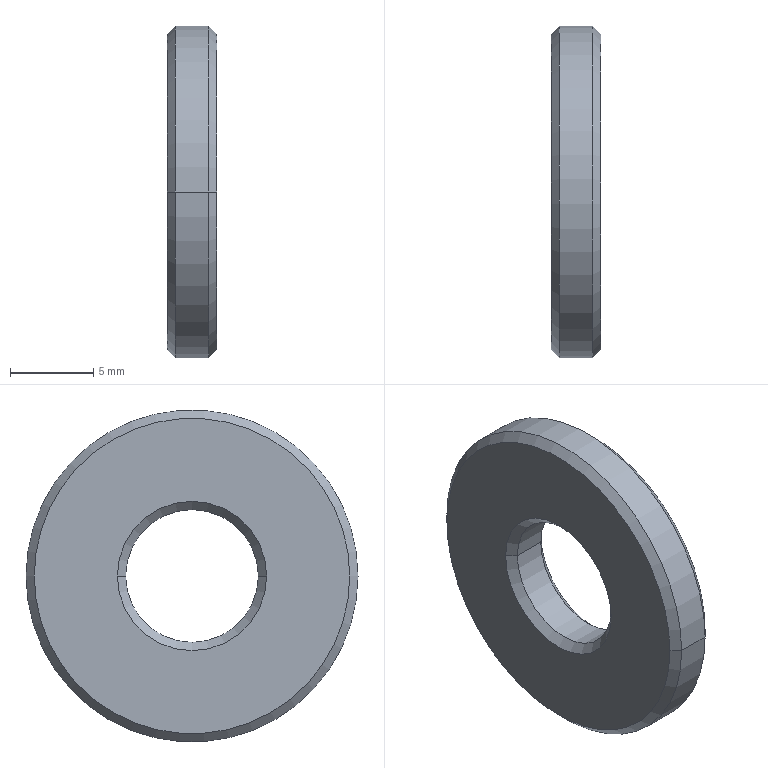Part | STEP file | wssm20_8_3_2_03 | 1 solid | 14 faces | box 3 x 20 x 20 mm | volume 769.69 mm3 | cone 8 | cylinder 4 | plane 2 | commonest cylinder face diameters 8 x2 20 x2
STEP:
#1=CARTESIAN_POINT('',(0.,0.,0.));
#2=DIRECTION('',(0.,0.,1.));
#3=DIRECTION('',(1.,0.,0.));
#4=AXIS2_PLACEMENT_3D('',#1,#2,#3);
#5=CARTESIAN_POINT('',(3.,9.5,0.));
#6=VERTEX_POINT('',#5);
#7=CARTESIAN_POINT('',(3.,-9.5,0.));
#8=VERTEX_POINT('',#7);
#9=CARTESIAN_POINT('',(3.,0.,0.));
#10=DIRECTION('',(1.,0.,0.));
#11=DIRECTION('',(0.,-1.,0.));
#12=AXIS2_PLACEMENT_3D('',#9,#10,#11);
#13=CIRCLE('',#12,9.5);
#14=CARTESIAN_POINT('',(2.5,0.,0.));
#15=DIRECTION('',(-1.,0.,0.));
#16=DIRECTION('',(0.,-1.,0.));
#17=AXIS2_PLACEMENT_3D('',#14,#15,#16);
#18=CONICAL_SURFACE('',#17,10.,0.7854);
#19=CARTESIAN_POINT('',(6.283,-0.5));
#20=DIRECTION('',(-1.,0.));
#21=VECTOR('',#20,1.);
#22=LINE('',#19,#21);
#23=(GEOMETRIC_REPRESENTATION_CONTEXT(2)PARAMETRIC_REPRESENTATION_CONTEXT()REPRESENTATION_CONTEXT('',''));
#24=DEFINITIONAL_REPRESENTATION('',(#22),#23);
#25=PCURVE('',#18,#24);
#26=CARTESIAN_POINT('',(3.,-7.,0.));
#27=DIRECTION('',(1.,0.,0.));
#28=DIRECTION('',(0.,0.,-1.));
#29=AXIS2_PLACEMENT_3D('',#26,#27,#28);
#30=PLANE('',#29);
#31=CARTESIAN_POINT('',(0.,7.));
#32=DIRECTION('',(0.,-1.));
#33=AXIS2_PLACEMENT_2D('',#31,#32);
#34=CIRCLE('',#33,9.5);
#35=(GEOMETRIC_REPRESENTATION_CONTEXT(2)PARAMETRIC_REPRESENTATION_CONTEXT()REPRESENTATION_CONTEXT('',''));
#36=DEFINITIONAL_REPRESENTATION('',(#34),#35);
#37=PCURVE('',#30,#36);
#38=SURFACE_CURVE('',#13,(#25,#37),.PCURVE_S1.);
#39=EDGE_CURVE('',#6,#8,#38,.T.);
#40=ORIENTED_EDGE('',*,*,#39,.F.);
#41=CARTESIAN_POINT('',(2.5,10.,0.));
#42=VERTEX_POINT('',#41);
#43=CARTESIAN_POINT('',(2.5,10.,0.));
#44=DIRECTION('',(-0.7071,0.7071,0.));
#45=VECTOR('',#44,1.);
#46=LINE('',#43,#45);
#47=CARTESIAN_POINT('',(3.142,0.));
#48=DIRECTION('',(0.,1.));
#49=VECTOR('',#48,1.);
#50=LINE('',#47,#49);
#51=(GEOMETRIC_REPRESENTATION_CONTEXT(2)PARAMETRIC_REPRESENTATION_CONTEXT()REPRESENTATION_CONTEXT('',''));
#52=DEFINITIONAL_REPRESENTATION('',(#50),#51);
#53=PCURVE('',#18,#52);
#54=CARTESIAN_POINT('',(2.5,0.,0.));
#55=DIRECTION('',(-1.,0.,0.));
#56=DIRECTION('',(0.,-1.,0.));
#57=AXIS2_PLACEMENT_3D('',#54,#55,#56);
#58=CONICAL_SURFACE('',#57,10.,0.7854);
#59=CARTESIAN_POINT('',(3.142,0.));
#60=DIRECTION('',(0.,1.));
#61=VECTOR('',#60,1.);
#62=LINE('',#59,#61);
#63=(GEOMETRIC_REPRESENTATION_CONTEXT(2)PARAMETRIC_REPRESENTATION_CONTEXT()REPRESENTATION_CONTEXT('',''));
#64=DEFINITIONAL_REPRESENTATION('',(#62),#63);
#65=PCURVE('',#58,#64);
#66=SURFACE_CURVE('',#46,(#53,#65),.PCURVE_S1.);
#67=EDGE_CURVE('',#6,#42,#66,.T.);
#68=ORIENTED_EDGE('',*,*,#67,.T.);
#69=CARTESIAN_POINT('',(2.5,-10.,0.));
#70=VERTEX_POINT('',#69);
#71=CARTESIAN_POINT('',(2.5,0.,0.));
#72=DIRECTION('',(1.,0.,0.));
#73=DIRECTION('',(0.,-1.,0.));
#74=AXIS2_PLACEMENT_3D('',#71,#72,#73);
#75=CIRCLE('',#74,10.);
#76=CARTESIAN_POINT('',(6.283,0.));
#77=DIRECTION('',(-1.,0.));
#78=VECTOR('',#77,1.);
#79=LINE('',#76,#78);
#80=(GEOMETRIC_REPRESENTATION_CONTEXT(2)PARAMETRIC_REPRESENTATION_CONTEXT()REPRESENTATION_CONTEXT('',''));
#81=DEFINITIONAL_REPRESENTATION('',(#79),#80);
#82=PCURVE('',#18,#81);
#83=CARTESIAN_POINT('',(1.5,0.,0.));
#84=DIRECTION('',(-1.,0.,0.));
#85=DIRECTION('',(0.,-1.,0.));
#86=AXIS2_PLACEMENT_3D('',#83,#84,#85);
#87=CYLINDRICAL_SURFACE('',#86,10.);
#88=CARTESIAN_POINT('',(6.283,-1.));
#89=DIRECTION('',(-1.,0.));
#90=VECTOR('',#89,1.);
#91=LINE('',#88,#90);
#92=(GEOMETRIC_REPRESENTATION_CONTEXT(2)PARAMETRIC_REPRESENTATION_CONTEXT()REPRESENTATION_CONTEXT('',''));
#93=DEFINITIONAL_REPRESENTATION('',(#91),#92);
#94=PCURVE('',#87,#93);
#95=SURFACE_CURVE('',#75,(#82,#94),.PCURVE_S1.);
#96=EDGE_CURVE('',#42,#70,#95,.T.);
#97=ORIENTED_EDGE('',*,*,#96,.T.);
#98=CARTESIAN_POINT('',(2.5,-10.,0.));
#99=DIRECTION('',(-0.7071,-0.7071,0.));
#100=VECTOR('',#99,1.);
#101=LINE('',#98,#100);
#102=CARTESIAN_POINT('',(0.,0.));
#103=DIRECTION('',(0.,1.));
#104=VECTOR('',#103,1.);
#105=LINE('',#102,#104);
#106=(GEOMETRIC_REPRESENTATION_CONTEXT(2)PARAMETRIC_REPRESENTATION_CONTEXT()REPRESENTATION_CONTEXT('',''));
#107=DEFINITIONAL_REPRESENTATION('',(#105),#106);
#108=PCURVE('',#18,#107);
#109=CARTESIAN_POINT('',(6.283,0.));
#110=DIRECTION('',(0.,1.));
#111=VECTOR('',#110,1.);
#112=LINE('',#109,#111);
#113=(GEOMETRIC_REPRESENTATION_CONTEXT(2)PARAMETRIC_REPRESENTATION_CONTEXT()REPRESENTATION_CONTEXT('',''));
#114=DEFINITIONAL_REPRESENTATION('',(#112),#113);
#115=PCURVE('',#58,#114);
#116=SURFACE_CURVE('',#101,(#108,#115),.PCURVE_S1.);
#117=EDGE_CURVE('',#8,#70,#116,.T.);
#118=ORIENTED_EDGE('',*,*,#117,.F.);
#119=EDGE_LOOP('',(#40,#68,#97,#118));
#120=FACE_BOUND('',#119,.T.);
#121=ADVANCED_FACE('',(#120),#18,.T.);
#122=CARTESIAN_POINT('',(2.5,-4.,0.));
#123=VERTEX_POINT('',#122);
#124=CARTESIAN_POINT('',(2.5,0.,-4.));
#125=VERTEX_POINT('',#124);
#126=CARTESIAN_POINT('',(2.5,0.,0.));
#127=DIRECTION('',(1.,0.,0.));
#128=DIRECTION('',(0.,-1.,0.));
#129=AXIS2_PLACEMENT_3D('',#126,#127,#128);
#130=CIRCLE('',#129,4.);
#131=CARTESIAN_POINT('',(3.,0.,0.));
#132=DIRECTION('',(1.,0.,0.));
#133=DIRECTION('',(0.,0.,-1.));
#134=AXIS2_PLACEMENT_3D('',#131,#132,#133);
#135=CONICAL_SURFACE('',#134,4.5,0.7854);
#136=CARTESIAN_POINT('',(4.712,-0.5));
#137=DIRECTION('',(1.,0.));
#138=VECTOR('',#137,1.);
#139=LINE('',#136,#138);
#140=(GEOMETRIC_REPRESENTATION_CONTEXT(2)PARAMETRIC_REPRESENTATION_CONTEXT()REPRESENTATION_CONTEXT('',''));
#141=DEFINITIONAL_REPRESENTATION('',(#139),#140);
#142=PCURVE('',#135,#141);
#143=CARTESIAN_POINT('',(1.5,0.,0.));
#144=DIRECTION('',(-1.,0.,0.));
#145=DIRECTION('',(0.,-1.,0.));
#146=AXIS2_PLACEMENT_3D('',#143,#144,#145);
#147=CYLINDRICAL_SURFACE('',#146,4.);
#148=CARTESIAN_POINT('',(6.283,-1.));
#149=DIRECTION('',(-1.,0.));
#150=VECTOR('',#149,1.);
#151=LINE('',#148,#150);
#152=(GEOMETRIC_REPRESENTATION_CONTEXT(2)PARAMETRIC_REPRESENTATION_CONTEXT()REPRESENTATION_CONTEXT('',''));
#153=DEFINITIONAL_REPRESENTATION('',(#151),#152);
#154=PCURVE('',#147,#153);
#155=SURFACE_CURVE('',#130,(#142,#154),.PCURVE_S1.);
#156=EDGE_CURVE('',#123,#125,#155,.T.);
#157=ORIENTED_EDGE('',*,*,#156,.T.);
#158=CARTESIAN_POINT('',(3.,0.,-4.5));
#159=VERTEX_POINT('',#158);
#160=CARTESIAN_POINT('',(3.,0.,-4.5));
#161=DIRECTION('',(0.7071,0.,-0.7071));
#162=VECTOR('',#161,1.);
#163=LINE('',#160,#162);
#164=CARTESIAN_POINT('',(6.283,0.));
#165=DIRECTION('',(0.,1.));
#166=VECTOR('',#165,1.);
#167=LINE('',#164,#166);
#168=(GEOMETRIC_REPRESENTATION_CONTEXT(2)PARAMETRIC_REPRESENTATION_CONTEXT()REPRESENTATION_CONTEXT('',''));
#169=DEFINITIONAL_REPRESENTATION('',(#167),#168);
#170=PCURVE('',#135,#169);
#171=CARTESIAN_POINT('',(3.,0.,0.));
#172=DIRECTION('',(1.,0.,0.));
#173=DIRECTION('',(0.,0.,-1.));
#174=AXIS2_PLACEMENT_3D('',#171,#172,#173);
#175=CONICAL_SURFACE('',#174,4.5,0.7854);
#176=CARTESIAN_POINT('',(0.,0.));
#177=DIRECTION('',(0.,1.));
#178=VECTOR('',#177,1.);
#179=LINE('',#176,#178);
#180=(GEOMETRIC_REPRESENTATION_CONTEXT(2)PARAMETRIC_REPRESENTATION_CONTEXT()REPRESENTATION_CONTEXT('',''));
#181=DEFINITIONAL_REPRESENTATION('',(#179),#180);
#182=PCURVE('',#175,#181);
#183=SURFACE_CURVE('',#163,(#170,#182),.PCURVE_S1.);
#184=EDGE_CURVE('',#125,#159,#183,.T.);
#185=ORIENTED_EDGE('',*,*,#184,.T.);
#186=CARTESIAN_POINT('',(3.,0.,4.5));
#187=VERTEX_POINT('',#186);
#188=CARTESIAN_POINT('',(3.,0.,0.));
#189=DIRECTION('',(-1.,0.,0.));
#190=DIRECTION('',(0.,0.,-1.));
#191=AXIS2_PLACEMENT_3D('',#188,#189,#190);
#192=CIRCLE('',#191,4.5);
#193=CARTESIAN_POINT('',(6.283,0.));
#194=DIRECTION('',(-1.,0.));
#195=VECTOR('',#194,1.);
#196=LINE('',#193,#195);
#197=(GEOMETRIC_REPRESENTATION_CONTEXT(2)PARAMETRIC_REPRESENTATION_CONTEXT()REPRESENTATION_CONTEXT('',''));
#198=DEFINITIONAL_REPRESENTATION('',(#196),#197);
#199=PCURVE('',#135,#198);
#200=CARTESIAN_POINT('',(4.5,7.));
#201=CARTESIAN_POINT('',(4.5,-0.7942));
#202=CARTESIAN_POINT('',(-2.25,3.103));
#203=CARTESIAN_POINT('',(-9.,7.));
#204=CARTESIAN_POINT('',(-2.25,10.897));
#205=CARTESIAN_POINT('',(4.5,14.794));
#206=CARTESIAN_POINT('',(4.5,7.));
#207=(BOUNDED_CURVE()B_SPLINE_CURVE(2,(#200,#201,#202,#203,#204,#205,#206),.UNSPECIFIED.,.T.,.F.)B_SPLINE_CURVE_WITH_KNOTS((1,2,2,2,2,1),(-2.094,0.,2.094,4.189,6.283,8.378),.UNSPECIFIED.)CURVE()GEOMETRIC_REPRESENTATION_ITEM()RATIONAL_B_SPLINE_CURVE((1.,0.5,1.,0.5,1.,0.5,1.))REPRESENTATION_ITEM(''));
#208=(GEOMETRIC_REPRESENTATION_CONTEXT(2)PARAMETRIC_REPRESENTATION_CONTEXT()REPRESENTATION_CONTEXT('',''));
#209=DEFINITIONAL_REPRESENTATION('',(#207),#208);
#210=PCURVE('',#30,#209);
#211=SURFACE_CURVE('',#192,(#199,#210),.PCURVE_S1.);
#212=EDGE_CURVE('',#159,#187,#211,.T.);
#213=ORIENTED_EDGE('',*,*,#212,.T.);
#214=CARTESIAN_POINT('',(2.5,0.,4.));
#215=VERTEX_POINT('',#214);
#216=CARTESIAN_POINT('',(3.,0.,4.5));
#217=DIRECTION('',(0.7071,0.,0.7071));
#218=VECTOR('',#217,1.);
#219=LINE('',#216,#218);
#220=CARTESIAN_POINT('',(3.142,0.));
#221=DIRECTION('',(0.,1.));
#222=VECTOR('',#221,1.);
#223=LINE('',#220,#222);
#224=(GEOMETRIC_REPRESENTATION_CONTEXT(2)PARAMETRIC_REPRESENTATION_CONTEXT()REPRESENTATION_CONTEXT('',''));
#225=DEFINITIONAL_REPRESENTATION('',(#223),#224);
#226=PCURVE('',#135,#225);
#227=CARTESIAN_POINT('',(3.142,0.));
#228=DIRECTION('',(0.,1.));
#229=VECTOR('',#228,1.);
#230=LINE('',#227,#229);
#231=(GEOMETRIC_REPRESENTATION_CONTEXT(2)PARAMETRIC_REPRESENTATION_CONTEXT()REPRESENTATION_CONTEXT('',''));
#232=DEFINITIONAL_REPRESENTATION('',(#230),#231);
#233=PCURVE('',#175,#232);
#234=SURFACE_CURVE('',#219,(#226,#233),.PCURVE_S1.);
#235=EDGE_CURVE('',#215,#187,#234,.T.);
#236=ORIENTED_EDGE('',*,*,#235,.F.);
#237=CARTESIAN_POINT('',(2.5,0.,0.));
#238=DIRECTION('',(1.,0.,0.));
#239=DIRECTION('',(0.,-1.,0.));
#240=AXIS2_PLACEMENT_3D('',#237,#238,#239);
#241=CIRCLE('',#240,4.);
#242=CARTESIAN_POINT('',(-1.571,-0.5));
#243=DIRECTION('',(1.,0.));
#244=VECTOR('',#243,1.);
#245=LINE('',#242,#244);
#246=(GEOMETRIC_REPRESENTATION_CONTEXT(2)PARAMETRIC_REPRESENTATION_CONTEXT()REPRESENTATION_CONTEXT('',''));
#247=DEFINITIONAL_REPRESENTATION('',(#245),#246);
#248=PCURVE('',#135,#247);
#249=CARTESIAN_POINT('',(1.5,0.,0.));
#250=DIRECTION('',(-1.,0.,0.));
#251=DIRECTION('',(0.,-1.,0.));
#252=AXIS2_PLACEMENT_3D('',#249,#250,#251);
#253=CYLINDRICAL_SURFACE('',#252,4.);
#254=CARTESIAN_POINT('',(6.283,-1.));
#255=DIRECTION('',(-1.,0.));
#256=VECTOR('',#255,1.);
#257=LINE('',#254,#256);
#258=(GEOMETRIC_REPRESENTATION_CONTEXT(2)PARAMETRIC_REPRESENTATION_CONTEXT()REPRESENTATION_CONTEXT('',''));
#259=DEFINITIONAL_REPRESENTATION('',(#257),#258);
#260=PCURVE('',#253,#259);
#261=SURFACE_CURVE('',#241,(#248,#260),.PCURVE_S1.);
#262=EDGE_CURVE('',#215,#123,#261,.T.);
#263=ORIENTED_EDGE('',*,*,#262,.T.);
#264=EDGE_LOOP('',(#157,#185,#213,#236,#263));
#265=FACE_BOUND('',#264,.F.);
#266=ADVANCED_FACE('',(#265),#135,.F.);
#267=ORIENTED_EDGE('',*,*,#96,.F.);
#268=CARTESIAN_POINT('',(0.5,10.,0.));
#269=VERTEX_POINT('',#268);
#270=CARTESIAN_POINT('',(1.5,10.,0.));
#271=DIRECTION('',(-1.,0.,0.));
#272=VECTOR('',#271,1.);
#273=LINE('',#270,#272);
#274=CARTESIAN_POINT('',(3.142,0.));
#275=DIRECTION('',(0.,1.));
#276=VECTOR('',#275,1.);
#277=LINE('',#274,#276);
#278=(GEOMETRIC_REPRESENTATION_CONTEXT(2)PARAMETRIC_REPRESENTATION_CONTEXT()REPRESENTATION_CONTEXT('',''));
#279=DEFINITIONAL_REPRESENTATION('',(#277),#278);
#280=PCURVE('',#87,#279);
#281=CARTESIAN_POINT('',(1.5,0.,0.));
#282=DIRECTION('',(-1.,0.,0.));
#283=DIRECTION('',(0.,-1.,0.));
#284=AXIS2_PLACEMENT_3D('',#281,#282,#283);
#285=CYLINDRICAL_SURFACE('',#284,10.);
#286=CARTESIAN_POINT('',(3.142,0.));
#287=DIRECTION('',(0.,1.));
#288=VECTOR('',#287,1.);
#289=LINE('',#286,#288);
#290=(GEOMETRIC_REPRESENTATION_CONTEXT(2)PARAMETRIC_REPRESENTATION_CONTEXT()REPRESENTATION_CONTEXT('',''));
#291=DEFINITIONAL_REPRESENTATION('',(#289),#290);
#292=PCURVE('',#285,#291);
#293=SURFACE_CURVE('',#273,(#280,#292),.PCURVE_S1.);
#294=EDGE_CURVE('',#42,#269,#293,.T.);
#295=ORIENTED_EDGE('',*,*,#294,.T.);
#296=CARTESIAN_POINT('',(0.5,-10.,0.));
#297=VERTEX_POINT('',#296);
#298=CARTESIAN_POINT('',(0.5,0.,0.));
#299=DIRECTION('',(1.,0.,0.));
#300=DIRECTION('',(0.,-1.,0.));
#301=AXIS2_PLACEMENT_3D('',#298,#299,#300);
#302=CIRCLE('',#301,10.);
#303=CARTESIAN_POINT('',(6.283,1.));
#304=DIRECTION('',(-1.,0.));
#305=VECTOR('',#304,1.);
#306=LINE('',#303,#305);
#307=(GEOMETRIC_REPRESENTATION_CONTEXT(2)PARAMETRIC_REPRESENTATION_CONTEXT()REPRESENTATION_CONTEXT('',''));
#308=DEFINITIONAL_REPRESENTATION('',(#306),#307);
#309=PCURVE('',#87,#308);
#310=CARTESIAN_POINT('',(0.5,0.,0.));
#311=DIRECTION('',(1.,0.,0.));
#312=DIRECTION('',(0.,1.,0.));
#313=AXIS2_PLACEMENT_3D('',#310,#311,#312);
#314=CONICAL_SURFACE('',#313,10.,0.7854);
#315=CARTESIAN_POINT('',(-3.142,0.));
#316=DIRECTION('',(1.,0.));
#317=VECTOR('',#316,1.);
#318=LINE('',#315,#317);
#319=(GEOMETRIC_REPRESENTATION_CONTEXT(2)PARAMETRIC_REPRESENTATION_CONTEXT()REPRESENTATION_CONTEXT('',''));
#320=DEFINITIONAL_REPRESENTATION('',(#318),#319);
#321=PCURVE('',#314,#320);
#322=SURFACE_CURVE('',#302,(#309,#321),.PCURVE_S1.);
#323=EDGE_CURVE('',#269,#297,#322,.T.);
#324=ORIENTED_EDGE('',*,*,#323,.T.);
#325=CARTESIAN_POINT('',(1.5,-10.,0.));
#326=DIRECTION('',(-1.,0.,0.));
#327=VECTOR('',#326,1.);
#328=LINE('',#325,#327);
#329=CARTESIAN_POINT('',(0.,0.));
#330=DIRECTION('',(0.,1.));
#331=VECTOR('',#330,1.);
#332=LINE('',#329,#331);
#333=(GEOMETRIC_REPRESENTATION_CONTEXT(2)PARAMETRIC_REPRESENTATION_CONTEXT()REPRESENTATION_CONTEXT('',''));
#334=DEFINITIONAL_REPRESENTATION('',(#332),#333);
#335=PCURVE('',#87,#334);
#336=CARTESIAN_POINT('',(6.283,0.));
#337=DIRECTION('',(0.,1.));
#338=VECTOR('',#337,1.);
#339=LINE('',#336,#338);
#340=(GEOMETRIC_REPRESENTATION_CONTEXT(2)PARAMETRIC_REPRESENTATION_CONTEXT()REPRESENTATION_CONTEXT('',''));
#341=DEFINITIONAL_REPRESENTATION('',(#339),#340);
#342=PCURVE('',#285,#341);
#343=SURFACE_CURVE('',#328,(#335,#342),.PCURVE_S1.);
#344=EDGE_CURVE('',#70,#297,#343,.T.);
#345=ORIENTED_EDGE('',*,*,#344,.F.);
#346=EDGE_LOOP('',(#267,#295,#324,#345));
#347=FACE_BOUND('',#346,.T.);
#348=ADVANCED_FACE('',(#347),#87,.T.);
#349=CARTESIAN_POINT('',(0.5,-4.,0.));
#350=VERTEX_POINT('',#349);
#351=CARTESIAN_POINT('',(1.5,-4.,0.));
#352=DIRECTION('',(-1.,0.,0.));
#353=VECTOR('',#352,1.);
#354=LINE('',#351,#353);
#355=CARTESIAN_POINT('',(6.283,0.));
#356=DIRECTION('',(0.,1.));
#357=VECTOR('',#356,1.);
#358=LINE('',#355,#357);
#359=(GEOMETRIC_REPRESENTATION_CONTEXT(2)PARAMETRIC_REPRESENTATION_CONTEXT()REPRESENTATION_CONTEXT('',''));
#360=DEFINITIONAL_REPRESENTATION('',(#358),#359);
#361=PCURVE('',#147,#360);
#362=CARTESIAN_POINT('',(0.,0.));
#363=DIRECTION('',(0.,1.));
#364=VECTOR('',#363,1.);
#365=LINE('',#362,#364);
#366=(GEOMETRIC_REPRESENTATION_CONTEXT(2)PARAMETRIC_REPRESENTATION_CONTEXT()REPRESENTATION_CONTEXT('',''));
#367=DEFINITIONAL_REPRESENTATION('',(#365),#366);
#368=PCURVE('',#253,#367);
#369=SURFACE_CURVE('',#354,(#361,#368),.PCURVE_S1.);
#370=EDGE_CURVE('',#123,#350,#369,.T.);
#371=ORIENTED_EDGE('',*,*,#370,.T.);
#372=CARTESIAN_POINT('',(0.5,4.,0.));
#373=VERTEX_POINT('',#372);
#374=CARTESIAN_POINT('',(0.5,0.,0.));
#375=DIRECTION('',(1.,0.,0.));
#376=DIRECTION('',(0.,-1.,0.));
#377=AXIS2_PLACEMENT_3D('',#374,#375,#376);
#378=CIRCLE('',#377,4.);
#379=CARTESIAN_POINT('',(6.283,1.));
#380=DIRECTION('',(-1.,0.));
#381=VECTOR('',#380,1.);
#382=LINE('',#379,#381);
#383=(GEOMETRIC_REPRESENTATION_CONTEXT(2)PARAMETRIC_REPRESENTATION_CONTEXT()REPRESENTATION_CONTEXT('',''));
#384=DEFINITIONAL_REPRESENTATION('',(#382),#383);
#385=PCURVE('',#147,#384);
#386=CARTESIAN_POINT('',(0.,0.,0.));
#387=DIRECTION('',(-1.,0.,0.));
#388=DIRECTION('',(0.,-1.,0.));
#389=AXIS2_PLACEMENT_3D('',#386,#387,#388);
#390=CONICAL_SURFACE('',#389,4.5,0.7854);
#391=CARTESIAN_POINT('',(6.283,-0.5));
#392=DIRECTION('',(-1.,0.));
#393=VECTOR('',#392,1.);
#394=LINE('',#391,#393);
#395=(GEOMETRIC_REPRESENTATION_CONTEXT(2)PARAMETRIC_REPRESENTATION_CONTEXT()REPRESENTATION_CONTEXT('',''));
#396=DEFINITIONAL_REPRESENTATION('',(#394),#395);
#397=PCURVE('',#390,#396);
#398=SURFACE_CURVE('',#378,(#385,#397),.PCURVE_S1.);
#399=EDGE_CURVE('',#350,#373,#398,.T.);
#400=ORIENTED_EDGE('',*,*,#399,.T.);
#401=CARTESIAN_POINT('',(2.5,4.,0.));
#402=VERTEX_POINT('',#401);
#403=CARTESIAN_POINT('',(1.5,4.,0.));
#404=DIRECTION('',(-1.,0.,0.));
#405=VECTOR('',#404,1.);
#406=LINE('',#403,#405);
#407=CARTESIAN_POINT('',(3.142,0.));
#408=DIRECTION('',(0.,1.));
#409=VECTOR('',#408,1.);
#410=LINE('',#407,#409);
#411=(GEOMETRIC_REPRESENTATION_CONTEXT(2)PARAMETRIC_REPRESENTATION_CONTEXT()REPRESENTATION_CONTEXT('',''));
#412=DEFINITIONAL_REPRESENTATION('',(#410),#411);
#413=PCURVE('',#147,#412);
#414=CARTESIAN_POINT('',(3.142,0.));
#415=DIRECTION('',(0.,1.));
#416=VECTOR('',#415,1.);
#417=LINE('',#414,#416);
#418=(GEOMETRIC_REPRESENTATION_CONTEXT(2)PARAMETRIC_REPRESENTATION_CONTEXT()REPRESENTATION_CONTEXT('',''));
#419=DEFINITIONAL_REPRESENTATION('',(#417),#418);
#420=PCURVE('',#253,#419);
#421=SURFACE_CURVE('',#406,(#413,#420),.PCURVE_S1.);
#422=EDGE_CURVE('',#402,#373,#421,.T.);
#423=ORIENTED_EDGE('',*,*,#422,.F.);
#424=CARTESIAN_POINT('',(2.5,0.,0.));
#425=DIRECTION('',(1.,0.,0.));
#426=DIRECTION('',(0.,-1.,0.));
#427=AXIS2_PLACEMENT_3D('',#424,#425,#426);
#428=CIRCLE('',#427,4.);
#429=CARTESIAN_POINT('',(6.283,-1.));
#430=DIRECTION('',(-1.,0.));
#431=VECTOR('',#430,1.);
#432=LINE('',#429,#431);
#433=(GEOMETRIC_REPRESENTATION_CONTEXT(2)PARAMETRIC_REPRESENTATION_CONTEXT()REPRESENTATION_CONTEXT('',''));
#434=DEFINITIONAL_REPRESENTATION('',(#432),#433);
#435=PCURVE('',#147,#434);
#436=CARTESIAN_POINT('',(-1.571,-0.5));
#437=DIRECTION('',(1.,0.));
#438=VECTOR('',#437,1.);
#439=LINE('',#436,#438);
#440=(GEOMETRIC_REPRESENTATION_CONTEXT(2)PARAMETRIC_REPRESENTATION_CONTEXT()REPRESENTATION_CONTEXT('',''));
#441=DEFINITIONAL_REPRESENTATION('',(#439),#440);
#442=PCURVE('',#175,#441);
#443=SURFACE_CURVE('',#428,(#435,#442),.PCURVE_S1.);
#444=EDGE_CURVE('',#125,#402,#443,.T.);
#445=ORIENTED_EDGE('',*,*,#444,.F.);
#446=ORIENTED_EDGE('',*,*,#156,.F.);
#447=EDGE_LOOP('',(#371,#400,#423,#445,#446));
#448=FACE_BOUND('',#447,.F.);
#449=ADVANCED_FACE('',(#448),#147,.F.);
#450=CARTESIAN_POINT('',(0.,9.5,0.));
#451=VERTEX_POINT('',#450);
#452=CARTESIAN_POINT('',(0.,-9.5,0.));
#453=VERTEX_POINT('',#452);
#454=CARTESIAN_POINT('',(0.,0.,0.));
#455=DIRECTION('',(1.,0.,0.));
#456=DIRECTION('',(0.,1.,0.));
#457=AXIS2_PLACEMENT_3D('',#454,#455,#456);
#458=CIRCLE('',#457,9.5);
#459=CARTESIAN_POINT('',(0.,-0.5));
#460=DIRECTION('',(1.,0.));
#461=VECTOR('',#460,1.);
#462=LINE('',#459,#461);
#463=(GEOMETRIC_REPRESENTATION_CONTEXT(2)PARAMETRIC_REPRESENTATION_CONTEXT()REPRESENTATION_CONTEXT('',''));
#464=DEFINITIONAL_REPRESENTATION('',(#462),#463);
#465=PCURVE('',#314,#464);
#466=CARTESIAN_POINT('',(0.,-7.,0.));
#467=DIRECTION('',(-1.,0.,0.));
#468=DIRECTION('',(0.,-1.,0.));
#469=AXIS2_PLACEMENT_3D('',#466,#467,#468);
#470=PLANE('',#469);
#471=CARTESIAN_POINT('',(-16.5,0.));
#472=CARTESIAN_POINT('',(-16.5,16.454));
#473=CARTESIAN_POINT('',(-2.25,8.227));
#474=CARTESIAN_POINT('',(12.,0.));
#475=CARTESIAN_POINT('',(-2.25,-8.227));
#476=CARTESIAN_POINT('',(-16.5,-16.454));
#477=CARTESIAN_POINT('',(-16.5,0.));
#478=(BOUNDED_CURVE()B_SPLINE_CURVE(2,(#471,#472,#473,#474,#475,#476,#477),.UNSPECIFIED.,.T.,.F.)B_SPLINE_CURVE_WITH_KNOTS((1,2,2,2,2,1),(-2.094,0.,2.094,4.189,6.283,8.378),.UNSPECIFIED.)CURVE()GEOMETRIC_REPRESENTATION_ITEM()RATIONAL_B_SPLINE_CURVE((1.,0.5,1.,0.5,1.,0.5,1.))REPRESENTATION_ITEM(''));
#479=(GEOMETRIC_REPRESENTATION_CONTEXT(2)PARAMETRIC_REPRESENTATION_CONTEXT()REPRESENTATION_CONTEXT('',''));
#480=DEFINITIONAL_REPRESENTATION('',(#478),#479);
#481=PCURVE('',#470,#480);
#482=SURFACE_CURVE('',#458,(#465,#481),.PCURVE_S1.);
#483=EDGE_CURVE('',#451,#453,#482,.T.);
#484=ORIENTED_EDGE('',*,*,#483,.T.);
#485=CARTESIAN_POINT('',(0.5,-10.,0.));
#486=DIRECTION('',(0.7071,-0.7071,0.));
#487=VECTOR('',#486,1.);
#488=LINE('',#485,#487);
#489=CARTESIAN_POINT('',(3.142,0.));
#490=DIRECTION('',(0.,1.));
#491=VECTOR('',#490,1.);
#492=LINE('',#489,#491);
#493=(GEOMETRIC_REPRESENTATION_CONTEXT(2)PARAMETRIC_REPRESENTATION_CONTEXT()REPRESENTATION_CONTEXT('',''));
#494=DEFINITIONAL_REPRESENTATION('',(#492),#493);
#495=PCURVE('',#314,#494);
#496=CARTESIAN_POINT('',(0.5,0.,0.));
#497=DIRECTION('',(1.,0.,0.));
#498=DIRECTION('',(0.,1.,0.));
#499=AXIS2_PLACEMENT_3D('',#496,#497,#498);
#500=CONICAL_SURFACE('',#499,10.,0.7854);
#501=CARTESIAN_POINT('',(3.142,0.));
#502=DIRECTION('',(0.,1.));
#503=VECTOR('',#502,1.);
#504=LINE('',#501,#503);
#505=(GEOMETRIC_REPRESENTATION_CONTEXT(2)PARAMETRIC_REPRESENTATION_CONTEXT()REPRESENTATION_CONTEXT('',''));
#506=DEFINITIONAL_REPRESENTATION('',(#504),#505);
#507=PCURVE('',#500,#506);
#508=SURFACE_CURVE('',#488,(#495,#507),.PCURVE_S1.);
#509=EDGE_CURVE('',#453,#297,#508,.T.);
#510=ORIENTED_EDGE('',*,*,#509,.T.);
#511=ORIENTED_EDGE('',*,*,#323,.F.);
#512=CARTESIAN_POINT('',(0.5,10.,0.));
#513=DIRECTION('',(0.7071,0.7071,0.));
#514=VECTOR('',#513,1.);
#515=LINE('',#512,#514);
#516=CARTESIAN_POINT('',(0.,0.));
#517=DIRECTION('',(0.,1.));
#518=VECTOR('',#517,1.);
#519=LINE('',#516,#518);
#520=(GEOMETRIC_REPRESENTATION_CONTEXT(2)PARAMETRIC_REPRESENTATION_CONTEXT()REPRESENTATION_CONTEXT('',''));
#521=DEFINITIONAL_REPRESENTATION('',(#519),#520);
#522=PCURVE('',#314,#521);
#523=CARTESIAN_POINT('',(6.283,0.));
#524=DIRECTION('',(0.,1.));
#525=VECTOR('',#524,1.);
#526=LINE('',#523,#525);
#527=(GEOMETRIC_REPRESENTATION_CONTEXT(2)PARAMETRIC_REPRESENTATION_CONTEXT()REPRESENTATION_CONTEXT('',''));
#528=DEFINITIONAL_REPRESENTATION('',(#526),#527);
#529=PCURVE('',#500,#528);
#530=SURFACE_CURVE('',#515,(#522,#529),.PCURVE_S1.);
#531=EDGE_CURVE('',#451,#269,#530,.T.);
#532=ORIENTED_EDGE('',*,*,#531,.F.);
#533=EDGE_LOOP('',(#484,#510,#511,#532));
#534=FACE_BOUND('',#533,.T.);
#535=ADVANCED_FACE('',(#534),#314,.T.);
#536=CARTESIAN_POINT('',(0.,-4.5,0.));
#537=VERTEX_POINT('',#536);
#538=CARTESIAN_POINT('',(0.,-4.5,0.));
#539=DIRECTION('',(-0.7071,-0.7071,0.));
#540=VECTOR('',#539,1.);
#541=LINE('',#538,#540);
#542=CARTESIAN_POINT('',(6.283,0.));
#543=DIRECTION('',(0.,1.));
#544=VECTOR('',#543,1.);
#545=LINE('',#542,#544);
#546=(GEOMETRIC_REPRESENTATION_CONTEXT(2)PARAMETRIC_REPRESENTATION_CONTEXT()REPRESENTATION_CONTEXT('',''));
#547=DEFINITIONAL_REPRESENTATION('',(#545),#546);
#548=PCURVE('',#390,#547);
#549=CARTESIAN_POINT('',(0.,0.,0.));
#550=DIRECTION('',(-1.,0.,0.));
#551=DIRECTION('',(0.,-1.,0.));
#552=AXIS2_PLACEMENT_3D('',#549,#550,#551);
#553=CONICAL_SURFACE('',#552,4.5,0.7854);
#554=CARTESIAN_POINT('',(0.,0.));
#555=DIRECTION('',(0.,1.));
#556=VECTOR('',#555,1.);
#557=LINE('',#554,#556);
#558=(GEOMETRIC_REPRESENTATION_CONTEXT(2)PARAMETRIC_REPRESENTATION_CONTEXT()REPRESENTATION_CONTEXT('',''));
#559=DEFINITIONAL_REPRESENTATION('',(#557),#558);
#560=PCURVE('',#553,#559);
#561=SURFACE_CURVE('',#541,(#548,#560),.PCURVE_S1.);
#562=EDGE_CURVE('',#350,#537,#561,.T.);
#563=ORIENTED_EDGE('',*,*,#562,.T.);
#564=CARTESIAN_POINT('',(0.,4.5,0.));
#565=VERTEX_POINT('',#564);
#566=CARTESIAN_POINT('',(0.,0.,0.));
#567=DIRECTION('',(1.,0.,0.));
#568=DIRECTION('',(0.,-1.,0.));
#569=AXIS2_PLACEMENT_3D('',#566,#567,#568);
#570=CIRCLE('',#569,4.5);
#571=CARTESIAN_POINT('',(6.283,0.));
#572=DIRECTION('',(-1.,0.));
#573=VECTOR('',#572,1.);
#574=LINE('',#571,#573);
#575=(GEOMETRIC_REPRESENTATION_CONTEXT(2)PARAMETRIC_REPRESENTATION_CONTEXT()REPRESENTATION_CONTEXT('',''));
#576=DEFINITIONAL_REPRESENTATION('',(#574),#575);
#577=PCURVE('',#390,#576);
#578=CARTESIAN_POINT('',(-2.5,0.));
#579=CARTESIAN_POINT('',(-2.5,-7.794));
#580=CARTESIAN_POINT('',(-9.25,-3.897));
#581=CARTESIAN_POINT('',(-16.,0.));
#582=CARTESIAN_POINT('',(-9.25,3.897));
#583=CARTESIAN_POINT('',(-2.5,7.794));
#584=CARTESIAN_POINT('',(-2.5,0.));
#585=(BOUNDED_CURVE()B_SPLINE_CURVE(2,(#578,#579,#580,#581,#582,#583,#584),.UNSPECIFIED.,.T.,.F.)B_SPLINE_CURVE_WITH_KNOTS((1,2,2,2,2,1),(-2.094,0.,2.094,4.189,6.283,8.378),.UNSPECIFIED.)CURVE()GEOMETRIC_REPRESENTATION_ITEM()RATIONAL_B_SPLINE_CURVE((1.,0.5,1.,0.5,1.,0.5,1.))REPRESENTATION_ITEM(''));
#586=(GEOMETRIC_REPRESENTATION_CONTEXT(2)PARAMETRIC_REPRESENTATION_CONTEXT()REPRESENTATION_CONTEXT('',''));
#587=DEFINITIONAL_REPRESENTATION('',(#585),#586);
#588=PCURVE('',#470,#587);
#589=SURFACE_CURVE('',#570,(#577,#588),.PCURVE_S1.);
#590=EDGE_CURVE('',#537,#565,#589,.T.);
#591=ORIENTED_EDGE('',*,*,#590,.T.);
#592=CARTESIAN_POINT('',(0.,4.5,0.));
#593=DIRECTION('',(-0.7071,0.7071,0.));
#594=VECTOR('',#593,1.);
#595=LINE('',#592,#594);
#596=CARTESIAN_POINT('',(3.142,0.));
#597=DIRECTION('',(0.,1.));
#598=VECTOR('',#597,1.);
#599=LINE('',#596,#598);
#600=(GEOMETRIC_REPRESENTATION_CONTEXT(2)PARAMETRIC_REPRESENTATION_CONTEXT()REPRESENTATION_CONTEXT('',''));
#601=DEFINITIONAL_REPRESENTATION('',(#599),#600);
#602=PCURVE('',#390,#601);
#603=CARTESIAN_POINT('',(3.142,0.));
#604=DIRECTION('',(0.,1.));
#605=VECTOR('',#604,1.);
#606=LINE('',#603,#605);
#607=(GEOMETRIC_REPRESENTATION_CONTEXT(2)PARAMETRIC_REPRESENTATION_CONTEXT()REPRESENTATION_CONTEXT('',''));
#608=DEFINITIONAL_REPRESENTATION('',(#606),#607);
#609=PCURVE('',#553,#608);
#610=SURFACE_CURVE('',#595,(#602,#609),.PCURVE_S1.);
#611=EDGE_CURVE('',#373,#565,#610,.T.);
#612=ORIENTED_EDGE('',*,*,#611,.F.);
#613=ORIENTED_EDGE('',*,*,#399,.F.);
#614=EDGE_LOOP('',(#563,#591,#612,#613));
#615=FACE_BOUND('',#614,.F.);
#616=ADVANCED_FACE('',(#615),#390,.F.);
#617=CARTESIAN_POINT('',(3.,0.,0.));
#618=DIRECTION('',(1.,0.,0.));
#619=DIRECTION('',(0.,-1.,0.));
#620=AXIS2_PLACEMENT_3D('',#617,#618,#619);
#621=CIRCLE('',#620,9.5);
#622=CARTESIAN_POINT('',(0.,7.));
#623=DIRECTION('',(0.,-1.));
#624=AXIS2_PLACEMENT_2D('',#622,#623);
#625=CIRCLE('',#624,9.5);
#626=(GEOMETRIC_REPRESENTATION_CONTEXT(2)PARAMETRIC_REPRESENTATION_CONTEXT()REPRESENTATION_CONTEXT('',''));
#627=DEFINITIONAL_REPRESENTATION('',(#625),#626);
#628=PCURVE('',#30,#627);
#629=CARTESIAN_POINT('',(6.283,-0.5));
#630=DIRECTION('',(-1.,0.));
#631=VECTOR('',#630,1.);
#632=LINE('',#629,#631);
#633=(GEOMETRIC_REPRESENTATION_CONTEXT(2)PARAMETRIC_REPRESENTATION_CONTEXT()REPRESENTATION_CONTEXT('',''));
#634=DEFINITIONAL_REPRESENTATION('',(#632),#633);
#635=PCURVE('',#58,#634);
#636=SURFACE_CURVE('',#621,(#628,#635),.PCURVE_S1.);
#637=EDGE_CURVE('',#8,#6,#636,.T.);
#638=ORIENTED_EDGE('',*,*,#637,.T.);
#639=ORIENTED_EDGE('',*,*,#39,.T.);
#640=EDGE_LOOP('',(#638,#639));
#641=FACE_BOUND('',#640,.T.);
#642=ORIENTED_EDGE('',*,*,#212,.T.);
#643=CARTESIAN_POINT('',(3.,0.,0.));
#644=DIRECTION('',(-1.,0.,0.));
#645=DIRECTION('',(0.,0.,-1.));
#646=AXIS2_PLACEMENT_3D('',#643,#644,#645);
#647=CIRCLE('',#646,4.5);
#648=CARTESIAN_POINT('',(4.5,7.));
#649=CARTESIAN_POINT('',(4.5,-0.7942));
#650=CARTESIAN_POINT('',(-2.25,3.103));
#651=CARTESIAN_POINT('',(-9.,7.));
#652=CARTESIAN_POINT('',(-2.25,10.897));
#653=CARTESIAN_POINT('',(4.5,14.794));
#654=CARTESIAN_POINT('',(4.5,7.));
#655=(BOUNDED_CURVE()B_SPLINE_CURVE(2,(#648,#649,#650,#651,#652,#653,#654),.UNSPECIFIED.,.T.,.F.)B_SPLINE_CURVE_WITH_KNOTS((1,2,2,2,2,1),(-2.094,0.,2.094,4.189,6.283,8.378),.UNSPECIFIED.)CURVE()GEOMETRIC_REPRESENTATION_ITEM()RATIONAL_B_SPLINE_CURVE((1.,0.5,1.,0.5,1.,0.5,1.))REPRESENTATION_ITEM(''));
#656=(GEOMETRIC_REPRESENTATION_CONTEXT(2)PARAMETRIC_REPRESENTATION_CONTEXT()REPRESENTATION_CONTEXT('',''));
#657=DEFINITIONAL_REPRESENTATION('',(#655),#656);
#658=PCURVE('',#30,#657);
#659=CARTESIAN_POINT('',(6.283,0.));
#660=DIRECTION('',(-1.,0.));
#661=VECTOR('',#660,1.);
#662=LINE('',#659,#661);
#663=(GEOMETRIC_REPRESENTATION_CONTEXT(2)PARAMETRIC_REPRESENTATION_CONTEXT()REPRESENTATION_CONTEXT('',''));
#664=DEFINITIONAL_REPRESENTATION('',(#662),#663);
#665=PCURVE('',#175,#664);
#666=SURFACE_CURVE('',#647,(#658,#665),.PCURVE_S1.);
#667=EDGE_CURVE('',#187,#159,#666,.T.);
#668=ORIENTED_EDGE('',*,*,#667,.T.);
#669=EDGE_LOOP('',(#642,#668));
#670=FACE_BOUND('',#669,.T.);
#671=ADVANCED_FACE('',(#641,#670),#30,.T.);
#672=ORIENTED_EDGE('',*,*,#67,.F.);
#673=ORIENTED_EDGE('',*,*,#637,.F.);
#674=ORIENTED_EDGE('',*,*,#117,.T.);
#675=CARTESIAN_POINT('',(2.5,0.,0.));
#676=DIRECTION('',(1.,0.,0.));
#677=DIRECTION('',(0.,-1.,0.));
#678=AXIS2_PLACEMENT_3D('',#675,#676,#677);
#679=CIRCLE('',#678,10.);
#680=CARTESIAN_POINT('',(6.283,0.));
#681=DIRECTION('',(-1.,0.));
#682=VECTOR('',#681,1.);
#683=LINE('',#680,#682);
#684=(GEOMETRIC_REPRESENTATION_CONTEXT(2)PARAMETRIC_REPRESENTATION_CONTEXT()REPRESENTATION_CONTEXT('',''));
#685=DEFINITIONAL_REPRESENTATION('',(#683),#684);
#686=PCURVE('',#58,#685);
#687=CARTESIAN_POINT('',(6.283,-1.));
#688=DIRECTION('',(-1.,0.));
#689=VECTOR('',#688,1.);
#690=LINE('',#687,#689);
#691=(GEOMETRIC_REPRESENTATION_CONTEXT(2)PARAMETRIC_REPRESENTATION_CONTEXT()REPRESENTATION_CONTEXT('',''));
#692=DEFINITIONAL_REPRESENTATION('',(#690),#691);
#693=PCURVE('',#285,#692);
#694=SURFACE_CURVE('',#679,(#686,#693),.PCURVE_S1.);
#695=EDGE_CURVE('',#70,#42,#694,.T.);
#696=ORIENTED_EDGE('',*,*,#695,.T.);
#697=EDGE_LOOP('',(#672,#673,#674,#696));
#698=FACE_BOUND('',#697,.T.);
#699=ADVANCED_FACE('',(#698),#58,.T.);
#700=ORIENTED_EDGE('',*,*,#667,.T.);
#701=ORIENTED_EDGE('',*,*,#184,.F.);
#702=ORIENTED_EDGE('',*,*,#444,.T.);
#703=CARTESIAN_POINT('',(2.5,0.,0.));
#704=DIRECTION('',(1.,0.,0.));
#705=DIRECTION('',(0.,-1.,0.));
#706=AXIS2_PLACEMENT_3D('',#703,#704,#705);
#707=CIRCLE('',#706,4.);
#708=CARTESIAN_POINT('',(-1.571,-0.5));
#709=DIRECTION('',(1.,0.));
#710=VECTOR('',#709,1.);
#711=LINE('',#708,#710);
#712=(GEOMETRIC_REPRESENTATION_CONTEXT(2)PARAMETRIC_REPRESENTATION_CONTEXT()REPRESENTATION_CONTEXT('',''));
#713=DEFINITIONAL_REPRESENTATION('',(#711),#712);
#714=PCURVE('',#175,#713);
#715=CARTESIAN_POINT('',(6.283,-1.));
#716=DIRECTION('',(-1.,0.));
#717=VECTOR('',#716,1.);
#718=LINE('',#715,#717);
#719=(GEOMETRIC_REPRESENTATION_CONTEXT(2)PARAMETRIC_REPRESENTATION_CONTEXT()REPRESENTATION_CONTEXT('',''));
#720=DEFINITIONAL_REPRESENTATION('',(#718),#719);
#721=PCURVE('',#253,#720);
#722=SURFACE_CURVE('',#707,(#714,#721),.PCURVE_S1.);
#723=EDGE_CURVE('',#402,#215,#722,.T.);
#724=ORIENTED_EDGE('',*,*,#723,.T.);
#725=ORIENTED_EDGE('',*,*,#235,.T.);
#726=EDGE_LOOP('',(#700,#701,#702,#724,#725));
#727=FACE_BOUND('',#726,.F.);
#728=ADVANCED_FACE('',(#727),#175,.F.);
#729=ORIENTED_EDGE('',*,*,#294,.F.);
#730=ORIENTED_EDGE('',*,*,#695,.F.);
#731=ORIENTED_EDGE('',*,*,#344,.T.);
#732=CARTESIAN_POINT('',(0.5,0.,0.));
#733=DIRECTION('',(1.,0.,0.));
#734=DIRECTION('',(0.,-1.,0.));
#735=AXIS2_PLACEMENT_3D('',#732,#733,#734);
#736=CIRCLE('',#735,10.);
#737=CARTESIAN_POINT('',(6.283,1.));
#738=DIRECTION('',(-1.,0.));
#739=VECTOR('',#738,1.);
#740=LINE('',#737,#739);
#741=(GEOMETRIC_REPRESENTATION_CONTEXT(2)PARAMETRIC_REPRESENTATION_CONTEXT()REPRESENTATION_CONTEXT('',''));
#742=DEFINITIONAL_REPRESENTATION('',(#740),#741);
#743=PCURVE('',#285,#742);
#744=CARTESIAN_POINT('',(3.142,0.));
#745=DIRECTION('',(1.,0.));
#746=VECTOR('',#745,1.);
#747=LINE('',#744,#746);
#748=(GEOMETRIC_REPRESENTATION_CONTEXT(2)PARAMETRIC_REPRESENTATION_CONTEXT()REPRESENTATION_CONTEXT('',''));
#749=DEFINITIONAL_REPRESENTATION('',(#747),#748);
#750=PCURVE('',#500,#749);
#751=SURFACE_CURVE('',#736,(#743,#750),.PCURVE_S1.);
#752=EDGE_CURVE('',#297,#269,#751,.T.);
#753=ORIENTED_EDGE('',*,*,#752,.T.);
#754=EDGE_LOOP('',(#729,#730,#731,#753));
#755=FACE_BOUND('',#754,.T.);
#756=ADVANCED_FACE('',(#755),#285,.T.);
#757=CARTESIAN_POINT('',(0.5,0.,0.));
#758=DIRECTION('',(1.,0.,0.));
#759=DIRECTION('',(0.,-1.,0.));
#760=AXIS2_PLACEMENT_3D('',#757,#758,#759);
#761=CIRCLE('',#760,4.);
#762=CARTESIAN_POINT('',(6.283,1.));
#763=DIRECTION('',(-1.,0.));
#764=VECTOR('',#763,1.);
#765=LINE('',#762,#764);
#766=(GEOMETRIC_REPRESENTATION_CONTEXT(2)PARAMETRIC_REPRESENTATION_CONTEXT()REPRESENTATION_CONTEXT('',''));
#767=DEFINITIONAL_REPRESENTATION('',(#765),#766);
#768=PCURVE('',#253,#767);
#769=CARTESIAN_POINT('',(6.283,-0.5));
#770=DIRECTION('',(-1.,0.));
#771=VECTOR('',#770,1.);
#772=LINE('',#769,#771);
#773=(GEOMETRIC_REPRESENTATION_CONTEXT(2)PARAMETRIC_REPRESENTATION_CONTEXT()REPRESENTATION_CONTEXT('',''));
#774=DEFINITIONAL_REPRESENTATION('',(#772),#773);
#775=PCURVE('',#553,#774);
#776=SURFACE_CURVE('',#761,(#768,#775),.PCURVE_S1.);
#777=EDGE_CURVE('',#373,#350,#776,.T.);
#778=ORIENTED_EDGE('',*,*,#777,.T.);
#779=ORIENTED_EDGE('',*,*,#370,.F.);
#780=ORIENTED_EDGE('',*,*,#262,.F.);
#781=ORIENTED_EDGE('',*,*,#723,.F.);
#782=ORIENTED_EDGE('',*,*,#422,.T.);
#783=EDGE_LOOP('',(#778,#779,#780,#781,#782));
#784=FACE_BOUND('',#783,.F.);
#785=ADVANCED_FACE('',(#784),#253,.F.);
#786=ORIENTED_EDGE('',*,*,#509,.F.);
#787=CARTESIAN_POINT('',(0.,0.,0.));
#788=DIRECTION('',(1.,0.,0.));
#789=DIRECTION('',(0.,1.,0.));
#790=AXIS2_PLACEMENT_3D('',#787,#788,#789);
#791=CIRCLE('',#790,9.5);
#792=CARTESIAN_POINT('',(0.,-0.5));
#793=DIRECTION('',(1.,0.));
#794=VECTOR('',#793,1.);
#795=LINE('',#792,#794);
#796=(GEOMETRIC_REPRESENTATION_CONTEXT(2)PARAMETRIC_REPRESENTATION_CONTEXT()REPRESENTATION_CONTEXT('',''));
#797=DEFINITIONAL_REPRESENTATION('',(#795),#796);
#798=PCURVE('',#500,#797);
#799=CARTESIAN_POINT('',(-16.5,0.));
#800=CARTESIAN_POINT('',(-16.5,16.454));
#801=CARTESIAN_POINT('',(-2.25,8.227));
#802=CARTESIAN_POINT('',(12.,0.));
#803=CARTESIAN_POINT('',(-2.25,-8.227));
#804=CARTESIAN_POINT('',(-16.5,-16.454));
#805=CARTESIAN_POINT('',(-16.5,0.));
#806=(BOUNDED_CURVE()B_SPLINE_CURVE(2,(#799,#800,#801,#802,#803,#804,#805),.UNSPECIFIED.,.T.,.F.)B_SPLINE_CURVE_WITH_KNOTS((1,2,2,2,2,1),(-2.094,0.,2.094,4.189,6.283,8.378),.UNSPECIFIED.)CURVE()GEOMETRIC_REPRESENTATION_ITEM()RATIONAL_B_SPLINE_CURVE((1.,0.5,1.,0.5,1.,0.5,1.))REPRESENTATION_ITEM(''));
#807=(GEOMETRIC_REPRESENTATION_CONTEXT(2)PARAMETRIC_REPRESENTATION_CONTEXT()REPRESENTATION_CONTEXT('',''));
#808=DEFINITIONAL_REPRESENTATION('',(#806),#807);
#809=PCURVE('',#470,#808);
#810=SURFACE_CURVE('',#791,(#798,#809),.PCURVE_S1.);
#811=EDGE_CURVE('',#453,#451,#810,.T.);
#812=ORIENTED_EDGE('',*,*,#811,.T.);
#813=ORIENTED_EDGE('',*,*,#531,.T.);
#814=ORIENTED_EDGE('',*,*,#752,.F.);
#815=EDGE_LOOP('',(#786,#812,#813,#814));
#816=FACE_BOUND('',#815,.T.);
#817=ADVANCED_FACE('',(#816),#500,.T.);
#818=CARTESIAN_POINT('',(0.,0.,0.));
#819=DIRECTION('',(1.,0.,0.));
#820=DIRECTION('',(0.,-1.,0.));
#821=AXIS2_PLACEMENT_3D('',#818,#819,#820);
#822=CIRCLE('',#821,4.5);
#823=CARTESIAN_POINT('',(6.283,0.));
#824=DIRECTION('',(-1.,0.));
#825=VECTOR('',#824,1.);
#826=LINE('',#823,#825);
#827=(GEOMETRIC_REPRESENTATION_CONTEXT(2)PARAMETRIC_REPRESENTATION_CONTEXT()REPRESENTATION_CONTEXT('',''));
#828=DEFINITIONAL_REPRESENTATION('',(#826),#827);
#829=PCURVE('',#553,#828);
#830=CARTESIAN_POINT('',(-2.5,0.));
#831=CARTESIAN_POINT('',(-2.5,-7.794));
#832=CARTESIAN_POINT('',(-9.25,-3.897));
#833=CARTESIAN_POINT('',(-16.,0.));
#834=CARTESIAN_POINT('',(-9.25,3.897));
#835=CARTESIAN_POINT('',(-2.5,7.794));
#836=CARTESIAN_POINT('',(-2.5,0.));
#837=(BOUNDED_CURVE()B_SPLINE_CURVE(2,(#830,#831,#832,#833,#834,#835,#836),.UNSPECIFIED.,.T.,.F.)B_SPLINE_CURVE_WITH_KNOTS((1,2,2,2,2,1),(-2.094,0.,2.094,4.189,6.283,8.378),.UNSPECIFIED.)CURVE()GEOMETRIC_REPRESENTATION_ITEM()RATIONAL_B_SPLINE_CURVE((1.,0.5,1.,0.5,1.,0.5,1.))REPRESENTATION_ITEM(''));
#838=(GEOMETRIC_REPRESENTATION_CONTEXT(2)PARAMETRIC_REPRESENTATION_CONTEXT()REPRESENTATION_CONTEXT('',''));
#839=DEFINITIONAL_REPRESENTATION('',(#837),#838);
#840=PCURVE('',#470,#839);
#841=SURFACE_CURVE('',#822,(#829,#840),.PCURVE_S1.);
#842=EDGE_CURVE('',#565,#537,#841,.T.);
#843=ORIENTED_EDGE('',*,*,#842,.T.);
#844=ORIENTED_EDGE('',*,*,#562,.F.);
#845=ORIENTED_EDGE('',*,*,#777,.F.);
#846=ORIENTED_EDGE('',*,*,#611,.T.);
#847=EDGE_LOOP('',(#843,#844,#845,#846));
#848=FACE_BOUND('',#847,.F.);
#849=ADVANCED_FACE('',(#848),#553,.F.);
#850=ORIENTED_EDGE('',*,*,#590,.T.);
#851=ORIENTED_EDGE('',*,*,#842,.T.);
#852=EDGE_LOOP('',(#850,#851));
#853=FACE_BOUND('',#852,.T.);
#854=ORIENTED_EDGE('',*,*,#483,.F.);
#855=ORIENTED_EDGE('',*,*,#811,.F.);
#856=EDGE_LOOP('',(#854,#855));
#857=FACE_BOUND('',#856,.T.);
#858=ADVANCED_FACE('',(#853,#857),#470,.T.);
#859=CLOSED_SHELL('',(#121,#266,#348,#449,#535,#616,#671,#699,#728,#756,#785,#817,#849,#858));
#860=MANIFOLD_SOLID_BREP('',#859);
#861=(LENGTH_UNIT()NAMED_UNIT(*)SI_UNIT(.MILLI.,.METRE.));
#862=UNCERTAINTY_MEASURE_WITH_UNIT(LENGTH_MEASURE(0.0000001),#861,'','');
#863=(NAMED_UNIT(*)PLANE_ANGLE_UNIT()SI_UNIT($,.RADIAN.));
#864=(NAMED_UNIT(*)SI_UNIT($,.STERADIAN.)SOLID_ANGLE_UNIT());
#865=(GEOMETRIC_REPRESENTATION_CONTEXT(3)GLOBAL_UNCERTAINTY_ASSIGNED_CONTEXT((#862))GLOBAL_UNIT_ASSIGNED_CONTEXT((#861,#863,#864))REPRESENTATION_CONTEXT('',''));
#866=ADVANCED_BREP_SHAPE_REPRESENTATION('',(#4,#860),#865);